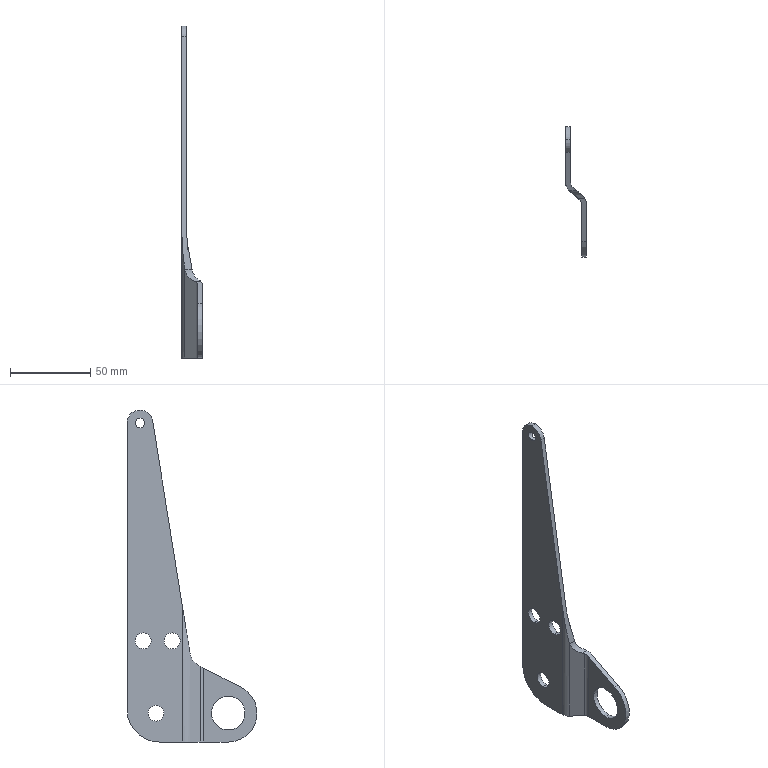Part | STEP file | 8XS174013 | 1 solid | 29 faces | box 13 x 81 x 207 mm | volume 21986 mm3 | cylinder 19 | plane 10 | commonest cylinder face diameters 10 x6 6 x4 12 x2 16 x2 21 x2 20 x1